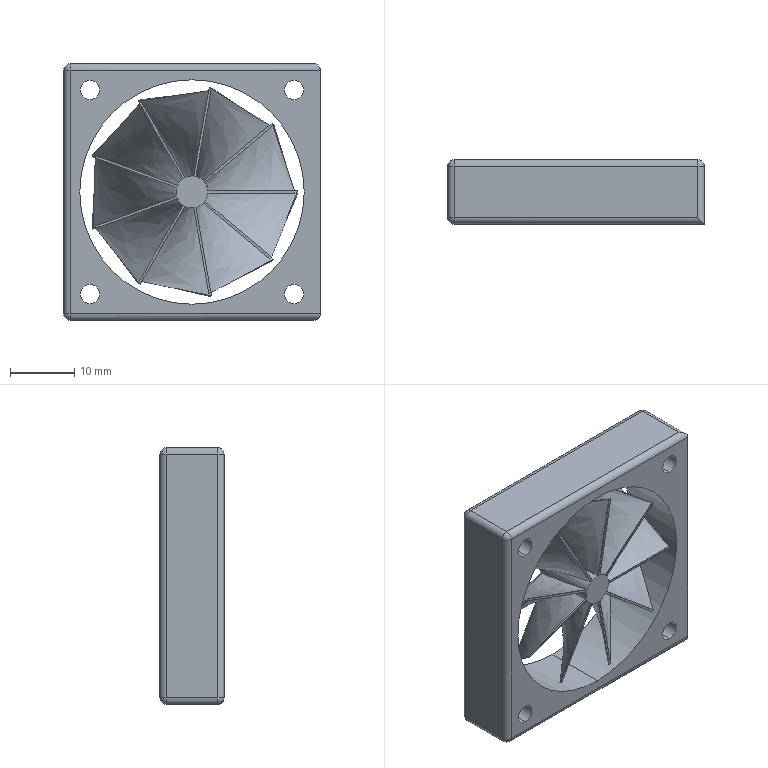Part | STEP file | Fan 40 | 2 solids | 127 faces | box 40 x 10 x 40 mm | volume 6606 mm3 | plane 62 | cylinder 32 | spline 27 | sphere 6 | commonest cylinder face diameters 2 x11 5 x11 3 x8 35 x2